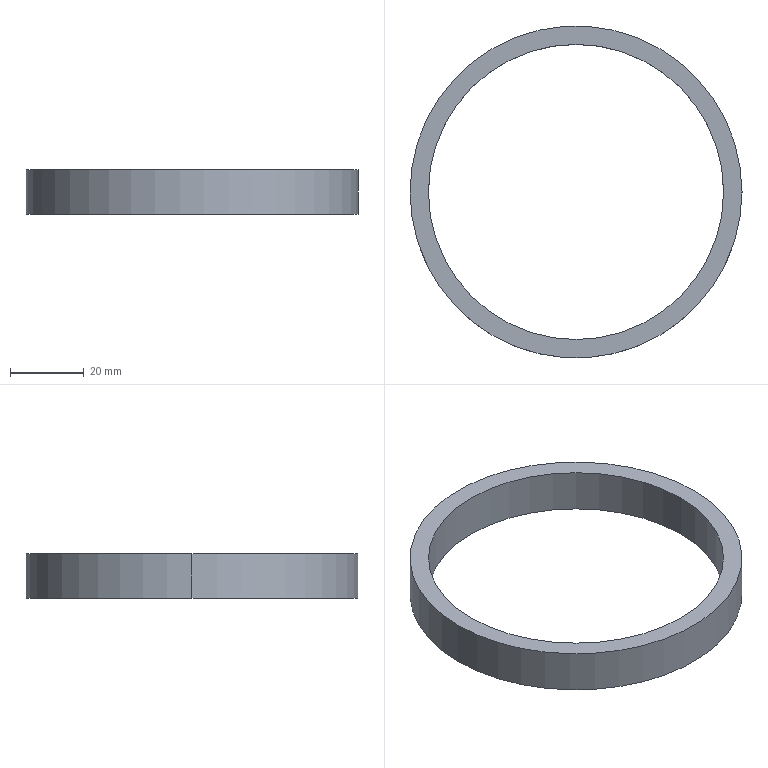Part | NX | features BREP 1 | 1 solid | 6 faces | box 90 x 90 x 12 mm | volume 16022 mm3 | cylinder 4 | plane 2 | commonest cylinder face diameters 80 x2 90 x2
STEP:
#1=CARTESIAN_POINT('',(-40.,0.,12.));
#2=VERTEX_POINT('',#1);
#3=CARTESIAN_POINT('',(40.,0.,12.));
#4=VERTEX_POINT('',#3);
#5=CARTESIAN_POINT('',(0.,0.,12.));
#6=DIRECTION('',(0.,0.,1.));
#7=DIRECTION('',(1.,0.,0.));
#8=AXIS2_PLACEMENT_3D('',#5,#6,#7);
#9=CIRCLE('',#8,40.);
#10=EDGE_CURVE('',#2,#4,#9,.T.);
#11=ORIENTED_EDGE('',*,*,#10,.T.);
#12=CARTESIAN_POINT('',(40.,0.,0.));
#13=VERTEX_POINT('',#12);
#14=CARTESIAN_POINT('',(40.,0.,12.));
#15=DIRECTION('',(0.,0.,-1.));
#16=VECTOR('',#15,1000.);
#17=LINE('',#14,#16);
#18=EDGE_CURVE('',#13,#4,#17,.F.);
#19=ORIENTED_EDGE('',*,*,#18,.F.);
#20=CARTESIAN_POINT('',(-40.,0.,0.));
#21=VERTEX_POINT('',#20);
#22=CARTESIAN_POINT('',(0.,0.,0.));
#23=DIRECTION('',(0.,0.,1.));
#24=DIRECTION('',(1.,0.,0.));
#25=AXIS2_PLACEMENT_3D('',#22,#23,#24);
#26=CIRCLE('',#25,40.);
#27=EDGE_CURVE('',#21,#13,#26,.T.);
#28=ORIENTED_EDGE('',*,*,#27,.F.);
#29=CARTESIAN_POINT('',(-40.,0.,12.));
#30=DIRECTION('',(0.,0.,-1.));
#31=VECTOR('',#30,1000.);
#32=LINE('',#29,#31);
#33=EDGE_CURVE('',#21,#2,#32,.F.);
#34=ORIENTED_EDGE('',*,*,#33,.T.);
#35=EDGE_LOOP('',(#11,#19,#28,#34));
#36=FACE_BOUND('',#35,.T.);
#37=CARTESIAN_POINT('',(0.,0.,12.));
#38=DIRECTION('',(0.,0.,-1.));
#39=DIRECTION('',(1.,0.,0.));
#40=AXIS2_PLACEMENT_3D('',#37,#38,#39);
#41=CYLINDRICAL_SURFACE('',#40,40.);
#42=ADVANCED_FACE('',(#36),#41,.F.);
#43=CARTESIAN_POINT('',(45.,0.,12.));
#44=VERTEX_POINT('',#43);
#45=CARTESIAN_POINT('',(-45.,0.,12.));
#46=VERTEX_POINT('',#45);
#47=CARTESIAN_POINT('',(0.,0.,12.));
#48=DIRECTION('',(0.,0.,1.));
#49=DIRECTION('',(1.,0.,0.));
#50=AXIS2_PLACEMENT_3D('',#47,#48,#49);
#51=CIRCLE('',#50,45.);
#52=EDGE_CURVE('',#44,#46,#51,.T.);
#53=ORIENTED_EDGE('',*,*,#52,.F.);
#54=CARTESIAN_POINT('',(45.,0.,0.));
#55=VERTEX_POINT('',#54);
#56=CARTESIAN_POINT('',(45.,0.,12.));
#57=DIRECTION('',(0.,0.,-1.));
#58=VECTOR('',#57,1000.);
#59=LINE('',#56,#58);
#60=EDGE_CURVE('',#55,#44,#59,.F.);
#61=ORIENTED_EDGE('',*,*,#60,.F.);
#62=CARTESIAN_POINT('',(-45.,0.,0.));
#63=VERTEX_POINT('',#62);
#64=CARTESIAN_POINT('',(0.,0.,0.));
#65=DIRECTION('',(0.,0.,1.));
#66=DIRECTION('',(1.,0.,0.));
#67=AXIS2_PLACEMENT_3D('',#64,#65,#66);
#68=CIRCLE('',#67,45.);
#69=EDGE_CURVE('',#55,#63,#68,.T.);
#70=ORIENTED_EDGE('',*,*,#69,.T.);
#71=CARTESIAN_POINT('',(-45.,0.,12.));
#72=DIRECTION('',(0.,0.,-1.));
#73=VECTOR('',#72,1000.);
#74=LINE('',#71,#73);
#75=EDGE_CURVE('',#63,#46,#74,.F.);
#76=ORIENTED_EDGE('',*,*,#75,.T.);
#77=EDGE_LOOP('',(#53,#61,#70,#76));
#78=FACE_BOUND('',#77,.T.);
#79=CARTESIAN_POINT('',(0.,0.,12.));
#80=DIRECTION('',(0.,0.,-1.));
#81=DIRECTION('',(1.,0.,0.));
#82=AXIS2_PLACEMENT_3D('',#79,#80,#81);
#83=CYLINDRICAL_SURFACE('',#82,45.);
#84=ADVANCED_FACE('',(#78),#83,.T.);
#85=CARTESIAN_POINT('',(0.,0.,12.));
#86=DIRECTION('',(0.,0.,1.));
#87=DIRECTION('',(1.,0.,0.));
#88=AXIS2_PLACEMENT_3D('',#85,#86,#87);
#89=CIRCLE('',#88,45.);
#90=EDGE_CURVE('',#46,#44,#89,.T.);
#91=ORIENTED_EDGE('',*,*,#90,.T.);
#92=ORIENTED_EDGE('',*,*,#52,.T.);
#93=EDGE_LOOP('',(#91,#92));
#94=FACE_BOUND('',#93,.T.);
#95=ORIENTED_EDGE('',*,*,#10,.F.);
#96=CARTESIAN_POINT('',(0.,0.,12.));
#97=DIRECTION('',(0.,0.,1.));
#98=DIRECTION('',(1.,0.,0.));
#99=AXIS2_PLACEMENT_3D('',#96,#97,#98);
#100=CIRCLE('',#99,40.);
#101=EDGE_CURVE('',#4,#2,#100,.T.);
#102=ORIENTED_EDGE('',*,*,#101,.F.);
#103=EDGE_LOOP('',(#95,#102));
#104=FACE_BOUND('',#103,.T.);
#105=CARTESIAN_POINT('',(0.,0.,12.));
#106=DIRECTION('',(0.,0.,1.));
#107=DIRECTION('',(-1.,0.,0.));
#108=AXIS2_PLACEMENT_3D('',#105,#106,#107);
#109=PLANE('',#108);
#110=ADVANCED_FACE('',(#94,#104),#109,.T.);
#111=CARTESIAN_POINT('',(0.,0.,0.));
#112=DIRECTION('',(0.,0.,1.));
#113=DIRECTION('',(1.,0.,0.));
#114=AXIS2_PLACEMENT_3D('',#111,#112,#113);
#115=CIRCLE('',#114,45.);
#116=EDGE_CURVE('',#63,#55,#115,.T.);
#117=ORIENTED_EDGE('',*,*,#116,.F.);
#118=ORIENTED_EDGE('',*,*,#69,.F.);
#119=EDGE_LOOP('',(#117,#118));
#120=FACE_BOUND('',#119,.T.);
#121=ORIENTED_EDGE('',*,*,#27,.T.);
#122=CARTESIAN_POINT('',(0.,0.,0.));
#123=DIRECTION('',(0.,0.,1.));
#124=DIRECTION('',(1.,0.,0.));
#125=AXIS2_PLACEMENT_3D('',#122,#123,#124);
#126=CIRCLE('',#125,40.);
#127=EDGE_CURVE('',#13,#21,#126,.T.);
#128=ORIENTED_EDGE('',*,*,#127,.T.);
#129=EDGE_LOOP('',(#121,#128));
#130=FACE_BOUND('',#129,.T.);
#131=CARTESIAN_POINT('',(0.,0.,0.));
#132=DIRECTION('',(0.,0.,1.));
#133=DIRECTION('',(-1.,0.,0.));
#134=AXIS2_PLACEMENT_3D('',#131,#132,#133);
#135=PLANE('',#134);
#136=ADVANCED_FACE('',(#120,#130),#135,.F.);
#137=ORIENTED_EDGE('',*,*,#60,.T.);
#138=ORIENTED_EDGE('',*,*,#90,.F.);
#139=ORIENTED_EDGE('',*,*,#75,.F.);
#140=ORIENTED_EDGE('',*,*,#116,.T.);
#141=EDGE_LOOP('',(#137,#138,#139,#140));
#142=FACE_BOUND('',#141,.T.);
#143=CARTESIAN_POINT('',(0.,0.,12.));
#144=DIRECTION('',(0.,0.,-1.));
#145=DIRECTION('',(1.,0.,0.));
#146=AXIS2_PLACEMENT_3D('',#143,#144,#145);
#147=CYLINDRICAL_SURFACE('',#146,45.);
#148=ADVANCED_FACE('',(#142),#147,.T.);
#149=ORIENTED_EDGE('',*,*,#18,.T.);
#150=ORIENTED_EDGE('',*,*,#101,.T.);
#151=ORIENTED_EDGE('',*,*,#33,.F.);
#152=ORIENTED_EDGE('',*,*,#127,.F.);
#153=EDGE_LOOP('',(#149,#150,#151,#152));
#154=FACE_BOUND('',#153,.T.);
#155=CARTESIAN_POINT('',(0.,0.,12.));
#156=DIRECTION('',(0.,0.,-1.));
#157=DIRECTION('',(1.,0.,0.));
#158=AXIS2_PLACEMENT_3D('',#155,#156,#157);
#159=CYLINDRICAL_SURFACE('',#158,40.);
#160=ADVANCED_FACE('',(#154),#159,.F.);
#161=CLOSED_SHELL('',(#42,#84,#110,#136,#148,#160));
#162=MANIFOLD_SOLID_BREP('',#161);
#163=(LENGTH_UNIT()NAMED_UNIT(*)SI_UNIT(.MILLI.,.METRE.));
#164=UNCERTAINTY_MEASURE_WITH_UNIT(LENGTH_MEASURE(0.00001),#163,'','');
#165=(NAMED_UNIT(*)PLANE_ANGLE_UNIT()SI_UNIT($,.RADIAN.));
#166=(NAMED_UNIT(*)SI_UNIT($,.STERADIAN.)SOLID_ANGLE_UNIT());
#167=(GEOMETRIC_REPRESENTATION_CONTEXT(3)GLOBAL_UNCERTAINTY_ASSIGNED_CONTEXT((#164))GLOBAL_UNIT_ASSIGNED_CONTEXT((#163,#165,#166))REPRESENTATION_CONTEXT('',''));
#168=ADVANCED_BREP_SHAPE_REPRESENTATION('',(#162),#167);